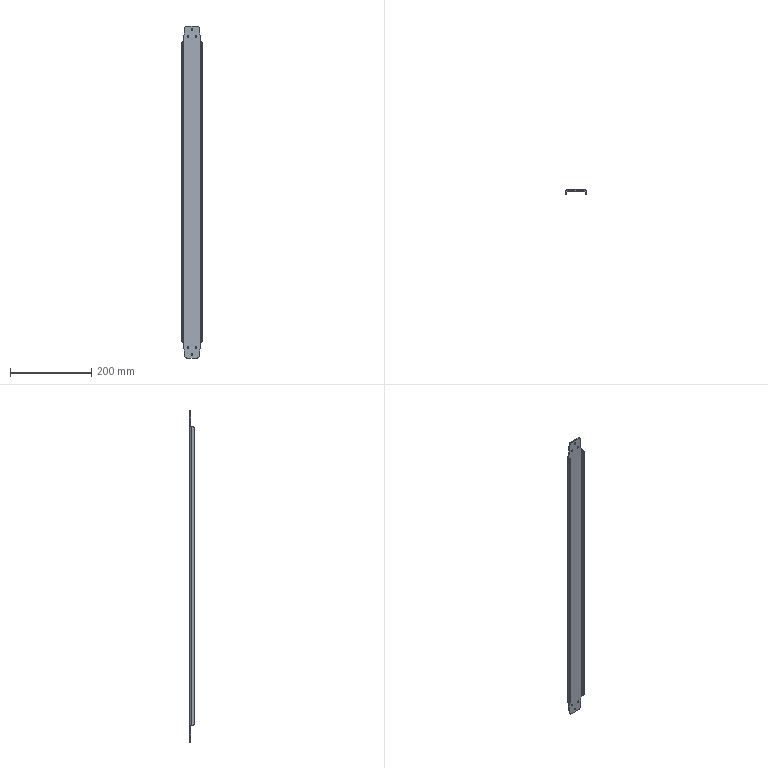Part | SolidWorks | features BaseBody 1 | 1 solid | 50 faces | box 50 x 10 x 815 mm | volume 124174 mm3 | cylinder 28 | plane 22 | commonest cylinder face diameters 4.5 x12 6 x10 10 x4 1 x2